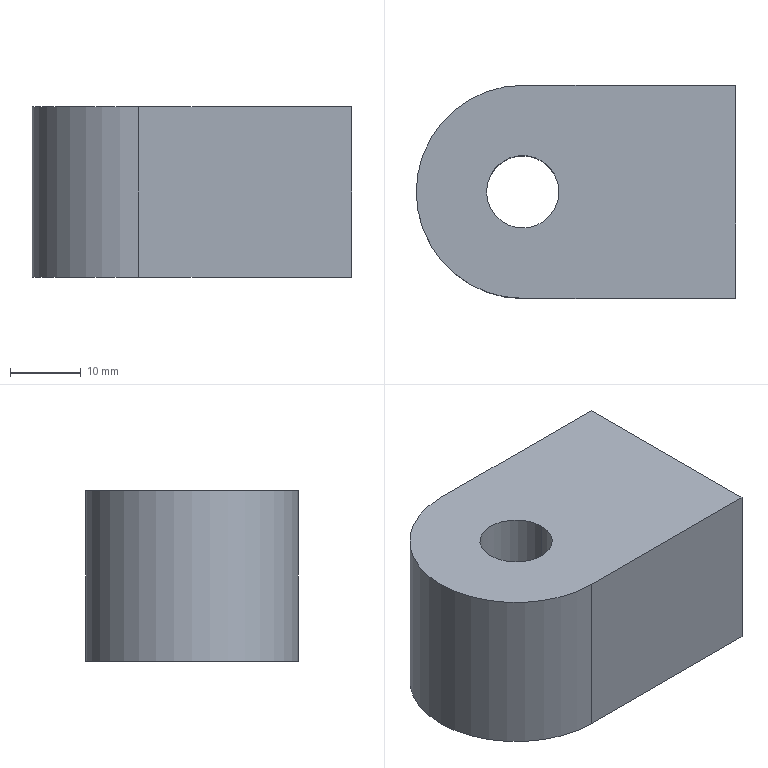Part | SolidWorks | features Extrusion 1 | 1 solid | 8 faces | box 45 x 30 x 24 mm | volume 28121 mm3 | plane 5 | cylinder 3 | commonest cylinder face diameters 10.2 x2 30 x1
STEP:
#1=CARTESIAN_POINT('',(-5.1,0.,-12.));
#2=VERTEX_POINT('',#1);
#3=CARTESIAN_POINT('',(5.1,0.,-12.));
#4=VERTEX_POINT('',#3);
#5=CARTESIAN_POINT('',(0.,0.,-12.));
#6=DIRECTION('',(0.,0.,1.));
#7=DIRECTION('',(1.,0.,0.));
#8=AXIS2_PLACEMENT_3D('',#5,#6,#7);
#9=CIRCLE('',#8,5.1);
#10=EDGE_CURVE('',#2,#4,#9,.T.);
#11=ORIENTED_EDGE('',*,*,#10,.F.);
#12=CARTESIAN_POINT('',(-5.1,0.,12.));
#13=VERTEX_POINT('',#12);
#14=CARTESIAN_POINT('',(-5.1,0.,-12.));
#15=DIRECTION('',(0.,0.,1.));
#16=VECTOR('',#15,1000.);
#17=LINE('',#14,#16);
#18=EDGE_CURVE('',#2,#13,#17,.T.);
#19=ORIENTED_EDGE('',*,*,#18,.T.);
#20=CARTESIAN_POINT('',(5.1,0.,12.));
#21=VERTEX_POINT('',#20);
#22=CARTESIAN_POINT('',(0.,0.,12.));
#23=DIRECTION('',(0.,0.,1.));
#24=DIRECTION('',(1.,0.,0.));
#25=AXIS2_PLACEMENT_3D('',#22,#23,#24);
#26=CIRCLE('',#25,5.1);
#27=EDGE_CURVE('',#13,#21,#26,.T.);
#28=ORIENTED_EDGE('',*,*,#27,.T.);
#29=CARTESIAN_POINT('',(5.1,0.,-12.));
#30=DIRECTION('',(0.,0.,1.));
#31=VECTOR('',#30,1000.);
#32=LINE('',#29,#31);
#33=EDGE_CURVE('',#4,#21,#32,.T.);
#34=ORIENTED_EDGE('',*,*,#33,.F.);
#35=EDGE_LOOP('',(#11,#19,#28,#34));
#36=FACE_OUTER_BOUND('',#35,.T.);
#37=CARTESIAN_POINT('',(0.,0.,-12.));
#38=DIRECTION('',(0.,0.,1.));
#39=DIRECTION('',(1.,0.,0.));
#40=AXIS2_PLACEMENT_3D('',#37,#38,#39);
#41=CYLINDRICAL_SURFACE('',#40,5.1);
#42=ADVANCED_FACE('',(#36),#41,.F.);
#43=CARTESIAN_POINT('',(0.,15.,12.));
#44=VERTEX_POINT('',#43);
#45=CARTESIAN_POINT('',(0.,-15.,12.));
#46=VERTEX_POINT('',#45);
#47=CARTESIAN_POINT('',(0.,0.,12.));
#48=DIRECTION('',(0.,0.,1.));
#49=DIRECTION('',(-1.,0.,0.));
#50=AXIS2_PLACEMENT_3D('',#47,#48,#49);
#51=CIRCLE('',#50,15.);
#52=EDGE_CURVE('',#44,#46,#51,.T.);
#53=ORIENTED_EDGE('',*,*,#52,.F.);
#54=CARTESIAN_POINT('',(0.,15.,-12.));
#55=VERTEX_POINT('',#54);
#56=CARTESIAN_POINT('',(0.,15.,-12.));
#57=DIRECTION('',(0.,0.,1.));
#58=VECTOR('',#57,1000.);
#59=LINE('',#56,#58);
#60=EDGE_CURVE('',#55,#44,#59,.T.);
#61=ORIENTED_EDGE('',*,*,#60,.F.);
#62=CARTESIAN_POINT('',(0.,-15.,-12.));
#63=VERTEX_POINT('',#62);
#64=CARTESIAN_POINT('',(0.,0.,-12.));
#65=DIRECTION('',(0.,0.,1.));
#66=DIRECTION('',(-1.,0.,0.));
#67=AXIS2_PLACEMENT_3D('',#64,#65,#66);
#68=CIRCLE('',#67,15.);
#69=EDGE_CURVE('',#55,#63,#68,.T.);
#70=ORIENTED_EDGE('',*,*,#69,.T.);
#71=CARTESIAN_POINT('',(0.,-15.,-12.));
#72=DIRECTION('',(0.,0.,1.));
#73=VECTOR('',#72,1000.);
#74=LINE('',#71,#73);
#75=EDGE_CURVE('',#63,#46,#74,.T.);
#76=ORIENTED_EDGE('',*,*,#75,.T.);
#77=EDGE_LOOP('',(#53,#61,#70,#76));
#78=FACE_OUTER_BOUND('',#77,.T.);
#79=CARTESIAN_POINT('',(0.,0.,-12.));
#80=DIRECTION('',(0.,0.,1.));
#81=DIRECTION('',(1.,0.,0.));
#82=AXIS2_PLACEMENT_3D('',#79,#80,#81);
#83=CYLINDRICAL_SURFACE('',#82,15.);
#84=ADVANCED_FACE('',(#78),#83,.T.);
#85=CARTESIAN_POINT('',(30.,15.,12.));
#86=VERTEX_POINT('',#85);
#87=CARTESIAN_POINT('',(0.,15.,12.));
#88=DIRECTION('',(-1.,0.,0.));
#89=VECTOR('',#88,1000.);
#90=LINE('',#87,#89);
#91=EDGE_CURVE('',#86,#44,#90,.T.);
#92=ORIENTED_EDGE('',*,*,#91,.F.);
#93=CARTESIAN_POINT('',(30.,15.,-12.));
#94=VERTEX_POINT('',#93);
#95=CARTESIAN_POINT('',(30.,15.,-12.));
#96=DIRECTION('',(0.,0.,1.));
#97=VECTOR('',#96,1000.);
#98=LINE('',#95,#97);
#99=EDGE_CURVE('',#94,#86,#98,.T.);
#100=ORIENTED_EDGE('',*,*,#99,.F.);
#101=CARTESIAN_POINT('',(0.,15.,-12.));
#102=DIRECTION('',(-1.,0.,0.));
#103=VECTOR('',#102,1000.);
#104=LINE('',#101,#103);
#105=EDGE_CURVE('',#94,#55,#104,.T.);
#106=ORIENTED_EDGE('',*,*,#105,.T.);
#107=ORIENTED_EDGE('',*,*,#60,.T.);
#108=EDGE_LOOP('',(#92,#100,#106,#107));
#109=FACE_OUTER_BOUND('',#108,.T.);
#110=CARTESIAN_POINT('',(0.,15.,-12.));
#111=DIRECTION('',(0.,1.,0.));
#112=DIRECTION('',(0.,0.,1.));
#113=AXIS2_PLACEMENT_3D('',#110,#111,#112);
#114=PLANE('',#113);
#115=ADVANCED_FACE('',(#109),#114,.T.);
#116=CARTESIAN_POINT('',(30.,-15.,12.));
#117=VERTEX_POINT('',#116);
#118=CARTESIAN_POINT('',(30.,15.,12.));
#119=DIRECTION('',(0.,1.,0.));
#120=VECTOR('',#119,1000.);
#121=LINE('',#118,#120);
#122=EDGE_CURVE('',#117,#86,#121,.T.);
#123=ORIENTED_EDGE('',*,*,#122,.F.);
#124=CARTESIAN_POINT('',(30.,-15.,-12.));
#125=VERTEX_POINT('',#124);
#126=CARTESIAN_POINT('',(30.,-15.,-12.));
#127=DIRECTION('',(0.,0.,1.));
#128=VECTOR('',#127,1000.);
#129=LINE('',#126,#128);
#130=EDGE_CURVE('',#125,#117,#129,.T.);
#131=ORIENTED_EDGE('',*,*,#130,.F.);
#132=CARTESIAN_POINT('',(30.,15.,-12.));
#133=DIRECTION('',(0.,1.,0.));
#134=VECTOR('',#133,1000.);
#135=LINE('',#132,#134);
#136=EDGE_CURVE('',#125,#94,#135,.T.);
#137=ORIENTED_EDGE('',*,*,#136,.T.);
#138=ORIENTED_EDGE('',*,*,#99,.T.);
#139=EDGE_LOOP('',(#123,#131,#137,#138));
#140=FACE_OUTER_BOUND('',#139,.T.);
#141=CARTESIAN_POINT('',(30.,15.,-12.));
#142=DIRECTION('',(1.,0.,0.));
#143=DIRECTION('',(0.,0.,-1.));
#144=AXIS2_PLACEMENT_3D('',#141,#142,#143);
#145=PLANE('',#144);
#146=ADVANCED_FACE('',(#140),#145,.T.);
#147=CARTESIAN_POINT('',(30.,-15.,12.));
#148=DIRECTION('',(1.,0.,0.));
#149=VECTOR('',#148,1000.);
#150=LINE('',#147,#149);
#151=EDGE_CURVE('',#46,#117,#150,.T.);
#152=ORIENTED_EDGE('',*,*,#151,.F.);
#153=ORIENTED_EDGE('',*,*,#75,.F.);
#154=CARTESIAN_POINT('',(30.,-15.,-12.));
#155=DIRECTION('',(1.,0.,0.));
#156=VECTOR('',#155,1000.);
#157=LINE('',#154,#156);
#158=EDGE_CURVE('',#63,#125,#157,.T.);
#159=ORIENTED_EDGE('',*,*,#158,.T.);
#160=ORIENTED_EDGE('',*,*,#130,.T.);
#161=EDGE_LOOP('',(#152,#153,#159,#160));
#162=FACE_OUTER_BOUND('',#161,.T.);
#163=CARTESIAN_POINT('',(30.,-15.,-12.));
#164=DIRECTION('',(0.,-1.,0.));
#165=DIRECTION('',(0.,0.,-1.));
#166=AXIS2_PLACEMENT_3D('',#163,#164,#165);
#167=PLANE('',#166);
#168=ADVANCED_FACE('',(#162),#167,.T.);
#169=CARTESIAN_POINT('',(0.,0.,-12.));
#170=DIRECTION('',(0.,0.,1.));
#171=DIRECTION('',(1.,0.,0.));
#172=AXIS2_PLACEMENT_3D('',#169,#170,#171);
#173=CIRCLE('',#172,5.1);
#174=EDGE_CURVE('',#4,#2,#173,.T.);
#175=ORIENTED_EDGE('',*,*,#174,.T.);
#176=ORIENTED_EDGE('',*,*,#10,.T.);
#177=EDGE_LOOP('',(#175,#176));
#178=FACE_BOUND('',#177,.T.);
#179=ORIENTED_EDGE('',*,*,#69,.F.);
#180=ORIENTED_EDGE('',*,*,#105,.F.);
#181=ORIENTED_EDGE('',*,*,#136,.F.);
#182=ORIENTED_EDGE('',*,*,#158,.F.);
#183=EDGE_LOOP('',(#179,#180,#181,#182));
#184=FACE_OUTER_BOUND('',#183,.T.);
#185=CARTESIAN_POINT('',(0.,0.,-12.));
#186=DIRECTION('',(0.,0.,-1.));
#187=DIRECTION('',(-1.,0.,0.));
#188=AXIS2_PLACEMENT_3D('',#185,#186,#187);
#189=PLANE('',#188);
#190=ADVANCED_FACE('',(#178,#184),#189,.T.);
#191=CARTESIAN_POINT('',(0.,0.,12.));
#192=DIRECTION('',(0.,0.,1.));
#193=DIRECTION('',(1.,0.,0.));
#194=AXIS2_PLACEMENT_3D('',#191,#192,#193);
#195=CIRCLE('',#194,5.1);
#196=EDGE_CURVE('',#21,#13,#195,.T.);
#197=ORIENTED_EDGE('',*,*,#196,.F.);
#198=ORIENTED_EDGE('',*,*,#27,.F.);
#199=EDGE_LOOP('',(#197,#198));
#200=FACE_BOUND('',#199,.T.);
#201=ORIENTED_EDGE('',*,*,#52,.T.);
#202=ORIENTED_EDGE('',*,*,#151,.T.);
#203=ORIENTED_EDGE('',*,*,#122,.T.);
#204=ORIENTED_EDGE('',*,*,#91,.T.);
#205=EDGE_LOOP('',(#201,#202,#203,#204));
#206=FACE_OUTER_BOUND('',#205,.T.);
#207=CARTESIAN_POINT('',(0.,0.,12.));
#208=DIRECTION('',(0.,0.,-1.));
#209=DIRECTION('',(-1.,0.,0.));
#210=AXIS2_PLACEMENT_3D('',#207,#208,#209);
#211=PLANE('',#210);
#212=ADVANCED_FACE('',(#200,#206),#211,.F.);
#213=ORIENTED_EDGE('',*,*,#18,.F.);
#214=ORIENTED_EDGE('',*,*,#174,.F.);
#215=ORIENTED_EDGE('',*,*,#33,.T.);
#216=ORIENTED_EDGE('',*,*,#196,.T.);
#217=EDGE_LOOP('',(#213,#214,#215,#216));
#218=FACE_OUTER_BOUND('',#217,.T.);
#219=CARTESIAN_POINT('',(0.,0.,-12.));
#220=DIRECTION('',(0.,0.,1.));
#221=DIRECTION('',(1.,0.,0.));
#222=AXIS2_PLACEMENT_3D('',#219,#220,#221);
#223=CYLINDRICAL_SURFACE('',#222,5.1);
#224=ADVANCED_FACE('',(#218),#223,.F.);
#225=CLOSED_SHELL('',(#42,#84,#115,#146,#168,#190,#212,#224));
#226=MANIFOLD_SOLID_BREP('',#225);
#227=CARTESIAN_POINT('',(0.,0.,0.));
#228=DIRECTION('',(0.,0.,1.));
#229=DIRECTION('',(1.,0.,0.));
#230=AXIS2_PLACEMENT_3D('',#227,#228,#229);
#231=(LENGTH_UNIT()NAMED_UNIT(*)SI_UNIT(.MILLI.,.METRE.));
#232=UNCERTAINTY_MEASURE_WITH_UNIT(LENGTH_MEASURE(0.00001),#231,'','');
#233=(NAMED_UNIT(*)PLANE_ANGLE_UNIT()SI_UNIT($,.RADIAN.));
#234=(NAMED_UNIT(*)SI_UNIT($,.STERADIAN.)SOLID_ANGLE_UNIT());
#235=(GEOMETRIC_REPRESENTATION_CONTEXT(3)GLOBAL_UNCERTAINTY_ASSIGNED_CONTEXT((#232))GLOBAL_UNIT_ASSIGNED_CONTEXT((#231,#233,#234))REPRESENTATION_CONTEXT('',''));
#236=ADVANCED_BREP_SHAPE_REPRESENTATION('',(#226,#230),#235);